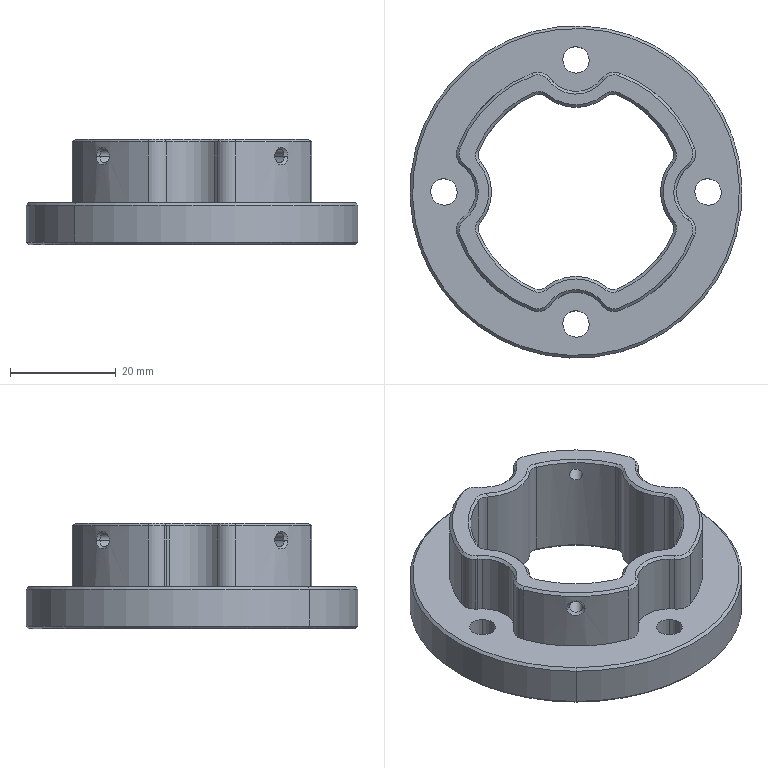NC program | NX | posted with a generic post | part box 62.9 x 62.9 x 20 mm
Lines 1 to 18 of 7695:
N10 G17 G21 G94 G90
(FLOOR_WALL , TOOL : D80)
N12 T19 M6
N14 G54
N16 G17 G0 G90 X-79.45 Y0. S6500 M3
N18 G43 Z30. H19
N20 Z3.
N22 G94 G1 Z0. F1500.
N24 X-76.45
N26 X76.45
N28 X79.45
N30 Z3.
N32 G0 Z30.
N34 M5